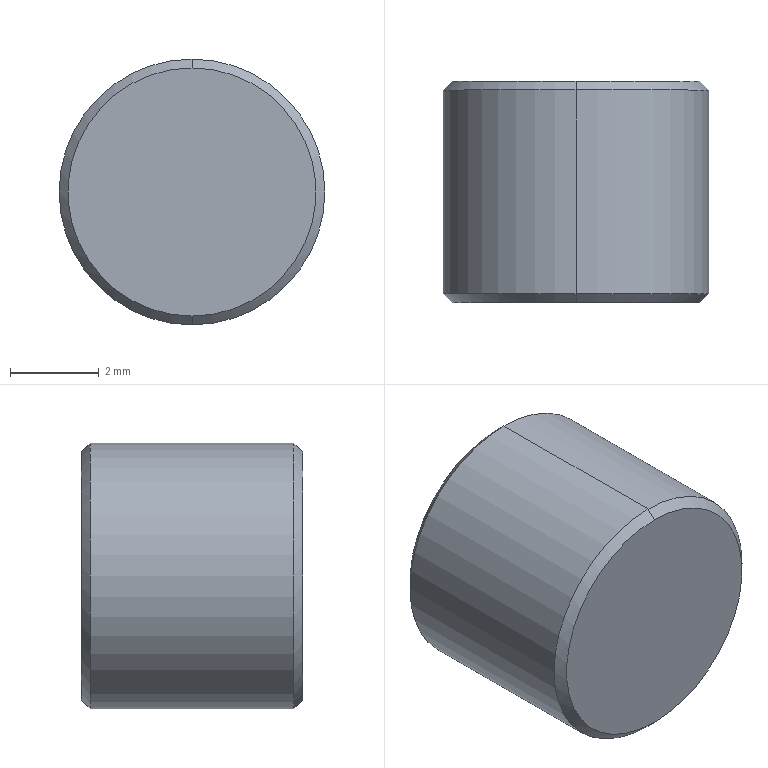Part | SolidWorks | features Chamfer 1, Extrusion 1 | 1 solid | 8 faces | box 6 x 5 x 6 mm | volume 140.634 mm3 | cone 4 | cylinder 2 | plane 2 | commonest cylinder face diameters 6 x2
STEP:
#1=CARTESIAN_POINT('',(0.,5.,2.8));
#2=VERTEX_POINT('',#1);
#3=CARTESIAN_POINT('',(0.,5.,-2.8));
#4=VERTEX_POINT('',#3);
#5=CARTESIAN_POINT('',(0.,5.,0.));
#6=DIRECTION('',(0.,1.,0.));
#7=DIRECTION('',(0.,0.,1.));
#8=AXIS2_PLACEMENT_3D('',#5,#6,#7);
#9=CIRCLE('',#8,2.8);
#10=EDGE_CURVE('',#2,#4,#9,.T.);
#11=ORIENTED_EDGE('',*,*,#10,.F.);
#12=CARTESIAN_POINT('',(0.,4.8,3.));
#13=VERTEX_POINT('',#12);
#14=CARTESIAN_POINT('',(0.,5.,2.8));
#15=DIRECTION('',(0.,-0.7071,0.7071));
#16=VECTOR('',#15,1000.);
#17=LINE('',#14,#16);
#18=EDGE_CURVE('',#2,#13,#17,.T.);
#19=ORIENTED_EDGE('',*,*,#18,.T.);
#20=CARTESIAN_POINT('',(0.,4.8,-3.));
#21=VERTEX_POINT('',#20);
#22=CARTESIAN_POINT('',(0.,4.8,0.));
#23=DIRECTION('',(0.,-1.,0.));
#24=DIRECTION('',(0.,0.,1.));
#25=AXIS2_PLACEMENT_3D('',#22,#23,#24);
#26=CIRCLE('',#25,3.);
#27=EDGE_CURVE('',#21,#13,#26,.T.);
#28=ORIENTED_EDGE('',*,*,#27,.F.);
#29=CARTESIAN_POINT('',(0.,5.,-2.8));
#30=DIRECTION('',(0.,-0.7071,-0.7071));
#31=VECTOR('',#30,1000.);
#32=LINE('',#29,#31);
#33=EDGE_CURVE('',#4,#21,#32,.T.);
#34=ORIENTED_EDGE('',*,*,#33,.F.);
#35=EDGE_LOOP('',(#11,#19,#28,#34));
#36=FACE_OUTER_BOUND('',#35,.T.);
#37=CARTESIAN_POINT('',(0.,5.,0.));
#38=DIRECTION('',(0.,-1.,0.));
#39=DIRECTION('',(0.,0.,-1.));
#40=AXIS2_PLACEMENT_3D('',#37,#38,#39);
#41=CONICAL_SURFACE('',#40,2.8,0.7854);
#42=ADVANCED_FACE('',(#36),#41,.T.);
#43=CARTESIAN_POINT('',(0.,0.,-2.8));
#44=VERTEX_POINT('',#43);
#45=CARTESIAN_POINT('',(0.,0.,2.8));
#46=VERTEX_POINT('',#45);
#47=CARTESIAN_POINT('',(0.,0.,0.));
#48=DIRECTION('',(0.,-1.,0.));
#49=DIRECTION('',(0.,0.,1.));
#50=AXIS2_PLACEMENT_3D('',#47,#48,#49);
#51=CIRCLE('',#50,2.8);
#52=EDGE_CURVE('',#44,#46,#51,.T.);
#53=ORIENTED_EDGE('',*,*,#52,.F.);
#54=CARTESIAN_POINT('',(0.,0.2,-3.));
#55=VERTEX_POINT('',#54);
#56=CARTESIAN_POINT('',(0.,0.2,-3.));
#57=DIRECTION('',(0.,0.7071,-0.7071));
#58=VECTOR('',#57,1000.);
#59=LINE('',#56,#58);
#60=EDGE_CURVE('',#44,#55,#59,.T.);
#61=ORIENTED_EDGE('',*,*,#60,.T.);
#62=CARTESIAN_POINT('',(0.,0.2,3.));
#63=VERTEX_POINT('',#62);
#64=CARTESIAN_POINT('',(0.,0.2,0.));
#65=DIRECTION('',(0.,1.,0.));
#66=DIRECTION('',(0.,0.,1.));
#67=AXIS2_PLACEMENT_3D('',#64,#65,#66);
#68=CIRCLE('',#67,3.);
#69=EDGE_CURVE('',#63,#55,#68,.T.);
#70=ORIENTED_EDGE('',*,*,#69,.F.);
#71=CARTESIAN_POINT('',(0.,0.2,3.));
#72=DIRECTION('',(0.,0.7071,0.7071));
#73=VECTOR('',#72,1000.);
#74=LINE('',#71,#73);
#75=EDGE_CURVE('',#46,#63,#74,.T.);
#76=ORIENTED_EDGE('',*,*,#75,.F.);
#77=EDGE_LOOP('',(#53,#61,#70,#76));
#78=FACE_OUTER_BOUND('',#77,.T.);
#79=CARTESIAN_POINT('',(0.,0.2,0.));
#80=DIRECTION('',(0.,1.,0.));
#81=DIRECTION('',(0.,0.,1.));
#82=AXIS2_PLACEMENT_3D('',#79,#80,#81);
#83=CONICAL_SURFACE('',#82,3.,0.7854);
#84=ADVANCED_FACE('',(#78),#83,.T.);
#85=ORIENTED_EDGE('',*,*,#27,.T.);
#86=CARTESIAN_POINT('',(0.,5.,3.));
#87=DIRECTION('',(0.,-1.,0.));
#88=VECTOR('',#87,1000.);
#89=LINE('',#86,#88);
#90=EDGE_CURVE('',#13,#63,#89,.T.);
#91=ORIENTED_EDGE('',*,*,#90,.T.);
#92=ORIENTED_EDGE('',*,*,#69,.T.);
#93=CARTESIAN_POINT('',(0.,5.,-3.));
#94=DIRECTION('',(0.,-1.,0.));
#95=VECTOR('',#94,1000.);
#96=LINE('',#93,#95);
#97=EDGE_CURVE('',#21,#55,#96,.T.);
#98=ORIENTED_EDGE('',*,*,#97,.F.);
#99=EDGE_LOOP('',(#85,#91,#92,#98));
#100=FACE_OUTER_BOUND('',#99,.T.);
#101=CARTESIAN_POINT('',(0.,5.,0.));
#102=DIRECTION('',(0.,-1.,0.));
#103=DIRECTION('',(0.,0.,-1.));
#104=AXIS2_PLACEMENT_3D('',#101,#102,#103);
#105=CYLINDRICAL_SURFACE('',#104,3.);
#106=ADVANCED_FACE('',(#100),#105,.T.);
#107=ORIENTED_EDGE('',*,*,#90,.F.);
#108=CARTESIAN_POINT('',(0.,4.8,0.));
#109=DIRECTION('',(0.,-1.,0.));
#110=DIRECTION('',(0.,0.,1.));
#111=AXIS2_PLACEMENT_3D('',#108,#109,#110);
#112=CIRCLE('',#111,3.);
#113=EDGE_CURVE('',#13,#21,#112,.T.);
#114=ORIENTED_EDGE('',*,*,#113,.T.);
#115=ORIENTED_EDGE('',*,*,#97,.T.);
#116=CARTESIAN_POINT('',(0.,0.2,0.));
#117=DIRECTION('',(0.,1.,0.));
#118=DIRECTION('',(0.,0.,1.));
#119=AXIS2_PLACEMENT_3D('',#116,#117,#118);
#120=CIRCLE('',#119,3.);
#121=EDGE_CURVE('',#55,#63,#120,.T.);
#122=ORIENTED_EDGE('',*,*,#121,.T.);
#123=EDGE_LOOP('',(#107,#114,#115,#122));
#124=FACE_OUTER_BOUND('',#123,.T.);
#125=CARTESIAN_POINT('',(0.,5.,0.));
#126=DIRECTION('',(0.,-1.,0.));
#127=DIRECTION('',(0.,0.,-1.));
#128=AXIS2_PLACEMENT_3D('',#125,#126,#127);
#129=CYLINDRICAL_SURFACE('',#128,3.);
#130=ADVANCED_FACE('',(#124),#129,.T.);
#131=CARTESIAN_POINT('',(0.,5.,0.));
#132=DIRECTION('',(0.,1.,0.));
#133=DIRECTION('',(0.,0.,1.));
#134=AXIS2_PLACEMENT_3D('',#131,#132,#133);
#135=CIRCLE('',#134,2.8);
#136=EDGE_CURVE('',#4,#2,#135,.T.);
#137=ORIENTED_EDGE('',*,*,#136,.T.);
#138=ORIENTED_EDGE('',*,*,#10,.T.);
#139=EDGE_LOOP('',(#137,#138));
#140=FACE_OUTER_BOUND('',#139,.T.);
#141=CARTESIAN_POINT('',(0.,5.,0.));
#142=DIRECTION('',(0.,1.,0.));
#143=DIRECTION('',(0.,0.,1.));
#144=AXIS2_PLACEMENT_3D('',#141,#142,#143);
#145=PLANE('',#144);
#146=ADVANCED_FACE('',(#140),#145,.T.);
#147=CARTESIAN_POINT('',(0.,0.,0.));
#148=DIRECTION('',(0.,-1.,0.));
#149=DIRECTION('',(0.,0.,1.));
#150=AXIS2_PLACEMENT_3D('',#147,#148,#149);
#151=CIRCLE('',#150,2.8);
#152=EDGE_CURVE('',#46,#44,#151,.T.);
#153=ORIENTED_EDGE('',*,*,#152,.T.);
#154=ORIENTED_EDGE('',*,*,#52,.T.);
#155=EDGE_LOOP('',(#153,#154));
#156=FACE_OUTER_BOUND('',#155,.T.);
#157=CARTESIAN_POINT('',(0.,0.,0.));
#158=DIRECTION('',(0.,1.,0.));
#159=DIRECTION('',(0.,0.,1.));
#160=AXIS2_PLACEMENT_3D('',#157,#158,#159);
#161=PLANE('',#160);
#162=ADVANCED_FACE('',(#156),#161,.F.);
#163=ORIENTED_EDGE('',*,*,#60,.F.);
#164=ORIENTED_EDGE('',*,*,#152,.F.);
#165=ORIENTED_EDGE('',*,*,#75,.T.);
#166=ORIENTED_EDGE('',*,*,#121,.F.);
#167=EDGE_LOOP('',(#163,#164,#165,#166));
#168=FACE_OUTER_BOUND('',#167,.T.);
#169=CARTESIAN_POINT('',(0.,0.2,0.));
#170=DIRECTION('',(0.,1.,0.));
#171=DIRECTION('',(0.,0.,1.));
#172=AXIS2_PLACEMENT_3D('',#169,#170,#171);
#173=CONICAL_SURFACE('',#172,3.,0.7854);
#174=ADVANCED_FACE('',(#168),#173,.T.);
#175=ORIENTED_EDGE('',*,*,#18,.F.);
#176=ORIENTED_EDGE('',*,*,#136,.F.);
#177=ORIENTED_EDGE('',*,*,#33,.T.);
#178=ORIENTED_EDGE('',*,*,#113,.F.);
#179=EDGE_LOOP('',(#175,#176,#177,#178));
#180=FACE_OUTER_BOUND('',#179,.T.);
#181=CARTESIAN_POINT('',(0.,5.,0.));
#182=DIRECTION('',(0.,-1.,0.));
#183=DIRECTION('',(0.,0.,-1.));
#184=AXIS2_PLACEMENT_3D('',#181,#182,#183);
#185=CONICAL_SURFACE('',#184,2.8,0.7854);
#186=ADVANCED_FACE('',(#180),#185,.T.);
#187=CLOSED_SHELL('',(#42,#84,#106,#130,#146,#162,#174,#186));
#188=MANIFOLD_SOLID_BREP('',#187);
#189=CARTESIAN_POINT('',(0.,0.,0.));
#190=DIRECTION('',(0.,0.,1.));
#191=DIRECTION('',(1.,0.,0.));
#192=AXIS2_PLACEMENT_3D('',#189,#190,#191);
#193=(LENGTH_UNIT()NAMED_UNIT(*)SI_UNIT(.MILLI.,.METRE.));
#194=UNCERTAINTY_MEASURE_WITH_UNIT(LENGTH_MEASURE(0.00001),#193,'','');
#195=(NAMED_UNIT(*)PLANE_ANGLE_UNIT()SI_UNIT($,.RADIAN.));
#196=(NAMED_UNIT(*)SI_UNIT($,.STERADIAN.)SOLID_ANGLE_UNIT());
#197=(GEOMETRIC_REPRESENTATION_CONTEXT(3)GLOBAL_UNCERTAINTY_ASSIGNED_CONTEXT((#194))GLOBAL_UNIT_ASSIGNED_CONTEXT((#193,#195,#196))REPRESENTATION_CONTEXT('',''));
#198=ADVANCED_BREP_SHAPE_REPRESENTATION('',(#188,#192),#197);